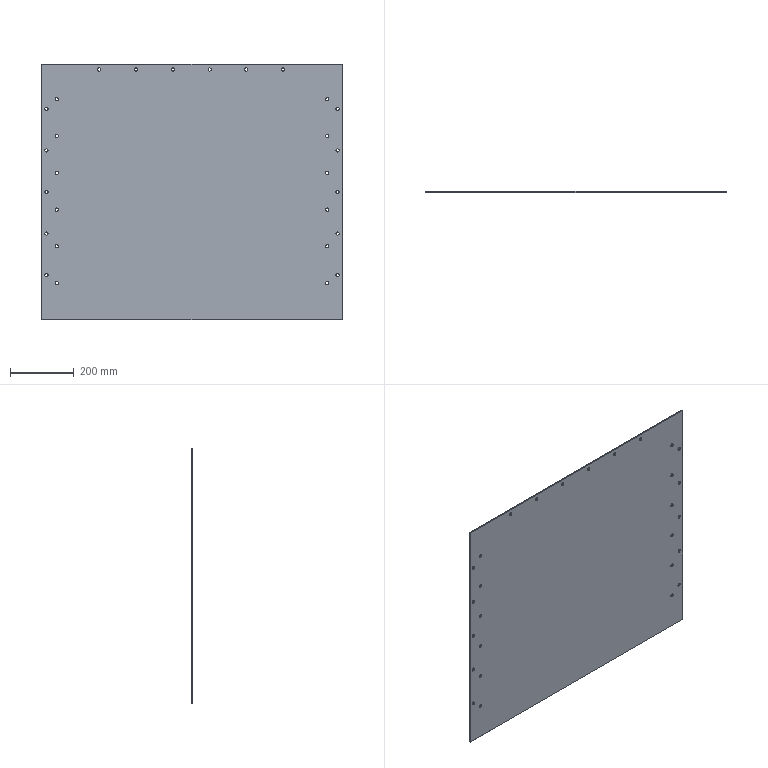Part | SolidWorks | features ICE 3, SMBaseFlange 2, FlatPattern 1, SheetMetal 1 | 1 solid | 62 faces | box 940 x 3 x 800 mm | volume 2249403 mm3 | cylinder 56 | plane 6 | commonest cylinder face diameters 10 x56